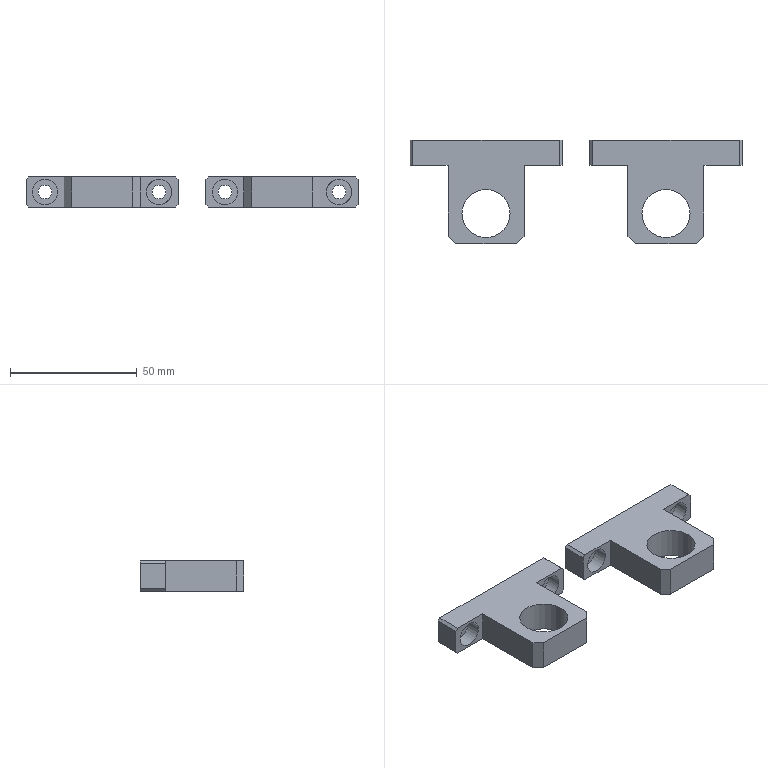Part | 2 solids | 46 faces | box 131 x 41 x 12 mm | volume 27460 mm3 | plane 36 | cylinder 10 | commonest cylinder face diameters 5.5 x4 10 x4 19 x2
STEP:
#1=CARTESIAN_POINT('',(22.5,18.2,5.));
#2=VERTEX_POINT('',#1);
#3=CARTESIAN_POINT('',(22.5,18.2,0.));
#4=DIRECTION('',(0.,-1.,0.));
#5=DIRECTION('',(0.,0.,1.));
#6=AXIS2_PLACEMENT_3D('',#3,#4,#5);
#7=CIRCLE('',#6,5.);
#8=EDGE_CURVE('',#2,#2,#7,.T.);
#9=ORIENTED_EDGE('',*,*,#8,.T.);
#10=EDGE_LOOP('',(#9));
#11=FACE_BOUND('',#10,.T.);
#12=CARTESIAN_POINT('',(22.5,18.2,2.75));
#13=VERTEX_POINT('',#12);
#14=CARTESIAN_POINT('',(22.5,18.2,0.));
#15=DIRECTION('',(0.,-1.,0.));
#16=DIRECTION('',(0.,0.,1.));
#17=AXIS2_PLACEMENT_3D('',#14,#15,#16);
#18=CIRCLE('',#17,2.75);
#19=EDGE_CURVE('',#13,#13,#18,.T.);
#20=ORIENTED_EDGE('',*,*,#19,.F.);
#21=EDGE_LOOP('',(#20));
#22=FACE_BOUND('',#21,.T.);
#23=CARTESIAN_POINT('',(-19.75,18.2,0.));
#24=DIRECTION('',(0.,1.,0.));
#25=DIRECTION('',(0.,0.,1.));
#26=AXIS2_PLACEMENT_3D('',#23,#24,#25);
#27=PLANE('',#26);
#28=ADVANCED_FACE('',(#11,#22),#27,.F.);
#29=CARTESIAN_POINT('',(-22.5,18.2,-5.));
#30=VERTEX_POINT('',#29);
#31=CARTESIAN_POINT('',(-22.5,18.2,0.));
#32=DIRECTION('',(0.,-1.,0.));
#33=DIRECTION('',(0.,0.,-1.));
#34=AXIS2_PLACEMENT_3D('',#31,#32,#33);
#35=CIRCLE('',#34,5.);
#36=EDGE_CURVE('',#30,#30,#35,.T.);
#37=ORIENTED_EDGE('',*,*,#36,.T.);
#38=EDGE_LOOP('',(#37));
#39=FACE_BOUND('',#38,.T.);
#40=CARTESIAN_POINT('',(-22.5,18.2,-2.75));
#41=VERTEX_POINT('',#40);
#42=CARTESIAN_POINT('',(-22.5,18.2,0.));
#43=DIRECTION('',(0.,-1.,0.));
#44=DIRECTION('',(0.,0.,-1.));
#45=AXIS2_PLACEMENT_3D('',#42,#43,#44);
#46=CIRCLE('',#45,2.75);
#47=EDGE_CURVE('',#41,#41,#46,.T.);
#48=ORIENTED_EDGE('',*,*,#47,.F.);
#49=EDGE_LOOP('',(#48));
#50=FACE_BOUND('',#49,.T.);
#51=CARTESIAN_POINT('',(-19.75,18.2,0.));
#52=DIRECTION('',(0.,1.,0.));
#53=DIRECTION('',(0.,0.,1.));
#54=AXIS2_PLACEMENT_3D('',#51,#52,#53);
#55=PLANE('',#54);
#56=ADVANCED_FACE('',(#39,#50),#55,.F.);
#57=CARTESIAN_POINT('',(29.,12.5,-6.));
#58=VERTEX_POINT('',#57);
#59=CARTESIAN_POINT('',(30.,12.5,-5.));
#60=VERTEX_POINT('',#59);
#61=CARTESIAN_POINT('',(5.5,12.5,-29.5));
#62=DIRECTION('',(0.7071,0.,0.7071));
#63=VECTOR('',#62,1000.);
#64=LINE('',#61,#63);
#65=EDGE_CURVE('',#58,#60,#64,.T.);
#66=ORIENTED_EDGE('',*,*,#65,.F.);
#67=CARTESIAN_POINT('',(29.,22.5,-6.));
#68=VERTEX_POINT('',#67);
#69=CARTESIAN_POINT('',(29.,0.,-6.));
#70=DIRECTION('',(0.,-1.,0.));
#71=VECTOR('',#70,1000.);
#72=LINE('',#69,#71);
#73=EDGE_CURVE('',#68,#58,#72,.T.);
#74=ORIENTED_EDGE('',*,*,#73,.F.);
#75=CARTESIAN_POINT('',(30.,22.5,-5.));
#76=VERTEX_POINT('',#75);
#77=CARTESIAN_POINT('',(30.,22.5,-5.));
#78=DIRECTION('',(-0.7071,0.,-0.7071));
#79=VECTOR('',#78,1000.);
#80=LINE('',#77,#79);
#81=EDGE_CURVE('',#76,#68,#80,.T.);
#82=ORIENTED_EDGE('',*,*,#81,.F.);
#83=CARTESIAN_POINT('',(30.,22.5,-5.));
#84=DIRECTION('',(0.,1.,0.));
#85=VECTOR('',#84,1000.);
#86=LINE('',#83,#85);
#87=EDGE_CURVE('',#60,#76,#86,.T.);
#88=ORIENTED_EDGE('',*,*,#87,.F.);
#89=EDGE_LOOP('',(#66,#74,#82,#88));
#90=FACE_BOUND('',#89,.T.);
#91=CARTESIAN_POINT('',(30.,22.5,-5.));
#92=DIRECTION('',(-0.7071,0.,0.7071));
#93=DIRECTION('',(0.,1.,0.));
#94=AXIS2_PLACEMENT_3D('',#91,#92,#93);
#95=PLANE('',#94);
#96=ADVANCED_FACE('',(#90),#95,.F.);
#97=CARTESIAN_POINT('',(30.,12.5,5.));
#98=VERTEX_POINT('',#97);
#99=CARTESIAN_POINT('',(29.,12.5,6.));
#100=VERTEX_POINT('',#99);
#101=CARTESIAN_POINT('',(-0.5,12.5,35.5));
#102=DIRECTION('',(-0.7071,0.,0.7071));
#103=VECTOR('',#102,1000.);
#104=LINE('',#101,#103);
#105=EDGE_CURVE('',#98,#100,#104,.T.);
#106=ORIENTED_EDGE('',*,*,#105,.F.);
#107=CARTESIAN_POINT('',(30.,22.5,5.));
#108=VERTEX_POINT('',#107);
#109=CARTESIAN_POINT('',(30.,12.5,5.));
#110=DIRECTION('',(0.,-1.,0.));
#111=VECTOR('',#110,1000.);
#112=LINE('',#109,#111);
#113=EDGE_CURVE('',#108,#98,#112,.T.);
#114=ORIENTED_EDGE('',*,*,#113,.F.);
#115=CARTESIAN_POINT('',(29.,22.5,6.));
#116=VERTEX_POINT('',#115);
#117=CARTESIAN_POINT('',(29.,22.5,6.));
#118=DIRECTION('',(0.7071,0.,-0.7071));
#119=VECTOR('',#118,1000.);
#120=LINE('',#117,#119);
#121=EDGE_CURVE('',#116,#108,#120,.T.);
#122=ORIENTED_EDGE('',*,*,#121,.F.);
#123=CARTESIAN_POINT('',(29.,22.5,6.));
#124=DIRECTION('',(0.,1.,0.));
#125=VECTOR('',#124,1000.);
#126=LINE('',#123,#125);
#127=EDGE_CURVE('',#100,#116,#126,.T.);
#128=ORIENTED_EDGE('',*,*,#127,.F.);
#129=EDGE_LOOP('',(#106,#114,#122,#128));
#130=FACE_BOUND('',#129,.T.);
#131=CARTESIAN_POINT('',(29.,0.,6.));
#132=DIRECTION('',(0.7071,0.,0.7071));
#133=DIRECTION('',(0.,-1.,0.));
#134=AXIS2_PLACEMENT_3D('',#131,#132,#133);
#135=PLANE('',#134);
#136=ADVANCED_FACE('',(#130),#135,.T.);
#137=CARTESIAN_POINT('',(-29.,22.5,-6.));
#138=VERTEX_POINT('',#137);
#139=CARTESIAN_POINT('',(-30.,22.5,-5.));
#140=VERTEX_POINT('',#139);
#141=CARTESIAN_POINT('',(-30.,22.5,-5.));
#142=DIRECTION('',(-0.7071,0.,0.7071));
#143=VECTOR('',#142,1000.);
#144=LINE('',#141,#143);
#145=EDGE_CURVE('',#138,#140,#144,.T.);
#146=ORIENTED_EDGE('',*,*,#145,.F.);
#147=CARTESIAN_POINT('',(-29.,12.5,-6.));
#148=VERTEX_POINT('',#147);
#149=CARTESIAN_POINT('',(-29.,0.,-6.));
#150=DIRECTION('',(0.,1.,0.));
#151=VECTOR('',#150,1000.);
#152=LINE('',#149,#151);
#153=EDGE_CURVE('',#148,#138,#152,.T.);
#154=ORIENTED_EDGE('',*,*,#153,.F.);
#155=CARTESIAN_POINT('',(-30.,12.5,-5.));
#156=VERTEX_POINT('',#155);
#157=CARTESIAN_POINT('',(-30.,12.5,-5.));
#158=DIRECTION('',(0.7071,0.,-0.7071));
#159=VECTOR('',#158,1000.);
#160=LINE('',#157,#159);
#161=EDGE_CURVE('',#156,#148,#160,.T.);
#162=ORIENTED_EDGE('',*,*,#161,.F.);
#163=CARTESIAN_POINT('',(-30.,22.5,-5.));
#164=DIRECTION('',(0.,-1.,0.));
#165=VECTOR('',#164,1000.);
#166=LINE('',#163,#165);
#167=EDGE_CURVE('',#140,#156,#166,.T.);
#168=ORIENTED_EDGE('',*,*,#167,.F.);
#169=EDGE_LOOP('',(#146,#154,#162,#168));
#170=FACE_BOUND('',#169,.T.);
#171=CARTESIAN_POINT('',(-30.,22.5,-5.));
#172=DIRECTION('',(0.7071,0.,0.7071));
#173=DIRECTION('',(0.,-1.,0.));
#174=AXIS2_PLACEMENT_3D('',#171,#172,#173);
#175=PLANE('',#174);
#176=ADVANCED_FACE('',(#170),#175,.F.);
#177=CARTESIAN_POINT('',(-30.,22.5,5.));
#178=VERTEX_POINT('',#177);
#179=CARTESIAN_POINT('',(-29.,22.5,6.));
#180=VERTEX_POINT('',#179);
#181=CARTESIAN_POINT('',(-29.,22.5,6.));
#182=DIRECTION('',(0.7071,0.,0.7071));
#183=VECTOR('',#182,1000.);
#184=LINE('',#181,#183);
#185=EDGE_CURVE('',#178,#180,#184,.T.);
#186=ORIENTED_EDGE('',*,*,#185,.F.);
#187=CARTESIAN_POINT('',(-30.,12.5,5.));
#188=VERTEX_POINT('',#187);
#189=CARTESIAN_POINT('',(-30.,22.5,5.));
#190=DIRECTION('',(0.,1.,0.));
#191=VECTOR('',#190,1000.);
#192=LINE('',#189,#191);
#193=EDGE_CURVE('',#188,#178,#192,.T.);
#194=ORIENTED_EDGE('',*,*,#193,.F.);
#195=CARTESIAN_POINT('',(-29.,12.5,6.));
#196=VERTEX_POINT('',#195);
#197=CARTESIAN_POINT('',(-29.,12.5,6.));
#198=DIRECTION('',(-0.7071,0.,-0.7071));
#199=VECTOR('',#198,1000.);
#200=LINE('',#197,#199);
#201=EDGE_CURVE('',#196,#188,#200,.T.);
#202=ORIENTED_EDGE('',*,*,#201,.F.);
#203=CARTESIAN_POINT('',(-29.,12.5,6.));
#204=DIRECTION('',(0.,-1.,0.));
#205=VECTOR('',#204,1000.);
#206=LINE('',#203,#205);
#207=EDGE_CURVE('',#180,#196,#206,.T.);
#208=ORIENTED_EDGE('',*,*,#207,.F.);
#209=EDGE_LOOP('',(#186,#194,#202,#208));
#210=FACE_BOUND('',#209,.T.);
#211=CARTESIAN_POINT('',(-29.,0.,6.));
#212=DIRECTION('',(-0.7071,0.,0.7071));
#213=DIRECTION('',(0.,1.,0.));
#214=AXIS2_PLACEMENT_3D('',#211,#212,#213);
#215=PLANE('',#214);
#216=ADVANCED_FACE('',(#210),#215,.T.);
#217=CARTESIAN_POINT('',(12.,-18.5,6.));
#218=VERTEX_POINT('',#217);
#219=CARTESIAN_POINT('',(15.,-15.5,6.));
#220=VERTEX_POINT('',#219);
#221=CARTESIAN_POINT('',(17.25,-13.25,6.));
#222=DIRECTION('',(0.7071,0.7071,0.));
#223=VECTOR('',#222,1000.);
#224=LINE('',#221,#223);
#225=EDGE_CURVE('',#218,#220,#224,.T.);
#226=ORIENTED_EDGE('',*,*,#225,.F.);
#227=CARTESIAN_POINT('',(12.,-18.5,-6.));
#228=VERTEX_POINT('',#227);
#229=CARTESIAN_POINT('',(12.,-18.5,6.));
#230=DIRECTION('',(0.,0.,1.));
#231=VECTOR('',#230,1000.);
#232=LINE('',#229,#231);
#233=EDGE_CURVE('',#228,#218,#232,.T.);
#234=ORIENTED_EDGE('',*,*,#233,.F.);
#235=CARTESIAN_POINT('',(15.,-15.5,-6.));
#236=VERTEX_POINT('',#235);
#237=CARTESIAN_POINT('',(15.,-15.5,-6.));
#238=DIRECTION('',(-0.7071,-0.7071,0.));
#239=VECTOR('',#238,1000.);
#240=LINE('',#237,#239);
#241=EDGE_CURVE('',#236,#228,#240,.T.);
#242=ORIENTED_EDGE('',*,*,#241,.F.);
#243=CARTESIAN_POINT('',(15.,-15.5,6.));
#244=DIRECTION('',(0.,0.,-1.));
#245=VECTOR('',#244,1000.);
#246=LINE('',#243,#245);
#247=EDGE_CURVE('',#220,#236,#246,.T.);
#248=ORIENTED_EDGE('',*,*,#247,.F.);
#249=EDGE_LOOP('',(#226,#234,#242,#248));
#250=FACE_BOUND('',#249,.T.);
#251=CARTESIAN_POINT('',(15.,-15.5,6.));
#252=DIRECTION('',(-0.7071,0.7071,0.));
#253=DIRECTION('',(0.,0.,-1.));
#254=AXIS2_PLACEMENT_3D('',#251,#252,#253);
#255=PLANE('',#254);
#256=ADVANCED_FACE('',(#250),#255,.F.);
#257=CARTESIAN_POINT('',(-15.,-15.5,6.));
#258=VERTEX_POINT('',#257);
#259=CARTESIAN_POINT('',(-12.,-18.5,6.));
#260=VERTEX_POINT('',#259);
#261=CARTESIAN_POINT('',(-17.25,-13.25,6.));
#262=DIRECTION('',(0.7071,-0.7071,0.));
#263=VECTOR('',#262,1000.);
#264=LINE('',#261,#263);
#265=EDGE_CURVE('',#258,#260,#264,.T.);
#266=ORIENTED_EDGE('',*,*,#265,.F.);
#267=CARTESIAN_POINT('',(-15.,-15.5,-6.));
#268=VERTEX_POINT('',#267);
#269=CARTESIAN_POINT('',(-15.,-15.5,6.));
#270=DIRECTION('',(0.,0.,1.));
#271=VECTOR('',#270,1000.);
#272=LINE('',#269,#271);
#273=EDGE_CURVE('',#268,#258,#272,.T.);
#274=ORIENTED_EDGE('',*,*,#273,.F.);
#275=CARTESIAN_POINT('',(-12.,-18.5,-6.));
#276=VERTEX_POINT('',#275);
#277=CARTESIAN_POINT('',(-12.,-18.5,-6.));
#278=DIRECTION('',(-0.7071,0.7071,0.));
#279=VECTOR('',#278,1000.);
#280=LINE('',#277,#279);
#281=EDGE_CURVE('',#276,#268,#280,.T.);
#282=ORIENTED_EDGE('',*,*,#281,.F.);
#283=CARTESIAN_POINT('',(-12.,-18.5,6.));
#284=DIRECTION('',(0.,0.,-1.));
#285=VECTOR('',#284,1000.);
#286=LINE('',#283,#285);
#287=EDGE_CURVE('',#260,#276,#286,.T.);
#288=ORIENTED_EDGE('',*,*,#287,.F.);
#289=EDGE_LOOP('',(#266,#274,#282,#288));
#290=FACE_BOUND('',#289,.T.);
#291=CARTESIAN_POINT('',(-12.,-18.5,6.));
#292=DIRECTION('',(0.7071,0.7071,0.));
#293=DIRECTION('',(0.,0.,-1.));
#294=AXIS2_PLACEMENT_3D('',#291,#292,#293);
#295=PLANE('',#294);
#296=ADVANCED_FACE('',(#290),#295,.F.);
#297=CARTESIAN_POINT('',(15.,12.5,6.));
#298=VERTEX_POINT('',#297);
#299=CARTESIAN_POINT('',(15.,-22.5,6.));
#300=DIRECTION('',(0.,1.,0.));
#301=VECTOR('',#300,1000.);
#302=LINE('',#299,#301);
#303=EDGE_CURVE('',#220,#298,#302,.T.);
#304=ORIENTED_EDGE('',*,*,#303,.F.);
#305=ORIENTED_EDGE('',*,*,#247,.T.);
#306=CARTESIAN_POINT('',(15.,12.5,-6.));
#307=VERTEX_POINT('',#306);
#308=CARTESIAN_POINT('',(15.,-22.5,-6.));
#309=DIRECTION('',(0.,1.,0.));
#310=VECTOR('',#309,1000.);
#311=LINE('',#308,#310);
#312=EDGE_CURVE('',#236,#307,#311,.T.);
#313=ORIENTED_EDGE('',*,*,#312,.T.);
#314=CARTESIAN_POINT('',(15.,12.5,6.));
#315=DIRECTION('',(0.,0.,-1.));
#316=VECTOR('',#315,1000.);
#317=LINE('',#314,#316);
#318=EDGE_CURVE('',#298,#307,#317,.T.);
#319=ORIENTED_EDGE('',*,*,#318,.F.);
#320=EDGE_LOOP('',(#304,#305,#313,#319));
#321=FACE_BOUND('',#320,.T.);
#322=CARTESIAN_POINT('',(15.,-22.5,6.));
#323=DIRECTION('',(-1.,0.,0.));
#324=DIRECTION('',(0.,0.,1.));
#325=AXIS2_PLACEMENT_3D('',#322,#323,#324);
#326=PLANE('',#325);
#327=ADVANCED_FACE('',(#321),#326,.F.);
#328=CARTESIAN_POINT('',(30.,12.5,6.));
#329=DIRECTION('',(0.,0.,-1.));
#330=VECTOR('',#329,1000.);
#331=LINE('',#328,#330);
#332=EDGE_CURVE('',#98,#60,#331,.T.);
#333=ORIENTED_EDGE('',*,*,#332,.F.);
#334=ORIENTED_EDGE('',*,*,#105,.T.);
#335=CARTESIAN_POINT('',(0.,12.5,6.));
#336=DIRECTION('',(1.,0.,0.));
#337=VECTOR('',#336,1000.);
#338=LINE('',#335,#337);
#339=EDGE_CURVE('',#298,#100,#338,.T.);
#340=ORIENTED_EDGE('',*,*,#339,.F.);
#341=ORIENTED_EDGE('',*,*,#318,.T.);
#342=CARTESIAN_POINT('',(-30.,12.5,-6.));
#343=DIRECTION('',(1.,0.,0.));
#344=VECTOR('',#343,1000.);
#345=LINE('',#342,#344);
#346=EDGE_CURVE('',#307,#58,#345,.T.);
#347=ORIENTED_EDGE('',*,*,#346,.T.);
#348=ORIENTED_EDGE('',*,*,#65,.T.);
#349=EDGE_LOOP('',(#333,#334,#340,#341,#347,#348));
#350=FACE_BOUND('',#349,.T.);
#351=CARTESIAN_POINT('',(17.5,12.5,0.));
#352=VERTEX_POINT('',#351);
#353=CARTESIAN_POINT('',(22.5,12.5,0.));
#354=DIRECTION('',(0.,-1.,0.));
#355=DIRECTION('',(-1.,0.,0.));
#356=AXIS2_PLACEMENT_3D('',#353,#354,#355);
#357=CIRCLE('',#356,5.);
#358=EDGE_CURVE('',#352,#352,#357,.T.);
#359=ORIENTED_EDGE('',*,*,#358,.F.);
#360=EDGE_LOOP('',(#359));
#361=FACE_BOUND('',#360,.T.);
#362=CARTESIAN_POINT('',(-30.,12.5,6.));
#363=DIRECTION('',(0.,1.,0.));
#364=DIRECTION('',(-1.,0.,0.));
#365=AXIS2_PLACEMENT_3D('',#362,#363,#364);
#366=PLANE('',#365);
#367=ADVANCED_FACE('',(#350,#361),#366,.F.);
#368=CARTESIAN_POINT('',(-15.,12.5,6.));
#369=VERTEX_POINT('',#368);
#370=CARTESIAN_POINT('',(-30.,12.5,6.));
#371=DIRECTION('',(1.,0.,0.));
#372=VECTOR('',#371,1000.);
#373=LINE('',#370,#372);
#374=EDGE_CURVE('',#196,#369,#373,.T.);
#375=ORIENTED_EDGE('',*,*,#374,.F.);
#376=ORIENTED_EDGE('',*,*,#201,.T.);
#377=CARTESIAN_POINT('',(-30.,12.5,6.));
#378=DIRECTION('',(0.,0.,-1.));
#379=VECTOR('',#378,1000.);
#380=LINE('',#377,#379);
#381=EDGE_CURVE('',#188,#156,#380,.T.);
#382=ORIENTED_EDGE('',*,*,#381,.T.);
#383=ORIENTED_EDGE('',*,*,#161,.T.);
#384=CARTESIAN_POINT('',(-15.,12.5,-6.));
#385=VERTEX_POINT('',#384);
#386=CARTESIAN_POINT('',(-30.,12.5,-6.));
#387=DIRECTION('',(1.,0.,0.));
#388=VECTOR('',#387,1000.);
#389=LINE('',#386,#388);
#390=EDGE_CURVE('',#148,#385,#389,.T.);
#391=ORIENTED_EDGE('',*,*,#390,.T.);
#392=CARTESIAN_POINT('',(-15.,12.5,6.));
#393=DIRECTION('',(0.,0.,-1.));
#394=VECTOR('',#393,1000.);
#395=LINE('',#392,#394);
#396=EDGE_CURVE('',#369,#385,#395,.T.);
#397=ORIENTED_EDGE('',*,*,#396,.F.);
#398=EDGE_LOOP('',(#375,#376,#382,#383,#391,#397));
#399=FACE_BOUND('',#398,.T.);
#400=CARTESIAN_POINT('',(-22.5,12.5,-5.));
#401=VERTEX_POINT('',#400);
#402=CARTESIAN_POINT('',(-22.5,12.5,0.));
#403=DIRECTION('',(0.,-1.,0.));
#404=DIRECTION('',(0.,0.,-1.));
#405=AXIS2_PLACEMENT_3D('',#402,#403,#404);
#406=CIRCLE('',#405,5.);
#407=EDGE_CURVE('',#401,#401,#406,.T.);
#408=ORIENTED_EDGE('',*,*,#407,.F.);
#409=EDGE_LOOP('',(#408));
#410=FACE_BOUND('',#409,.T.);
#411=CARTESIAN_POINT('',(-30.,12.5,6.));
#412=DIRECTION('',(0.,1.,0.));
#413=DIRECTION('',(-1.,0.,0.));
#414=AXIS2_PLACEMENT_3D('',#411,#412,#413);
#415=PLANE('',#414);
#416=ADVANCED_FACE('',(#399,#410),#415,.F.);
#417=CARTESIAN_POINT('',(-15.,-22.5,-6.));
#418=DIRECTION('',(0.,-1.,0.));
#419=VECTOR('',#418,1000.);
#420=LINE('',#417,#419);
#421=EDGE_CURVE('',#385,#268,#420,.T.);
#422=ORIENTED_EDGE('',*,*,#421,.T.);
#423=ORIENTED_EDGE('',*,*,#273,.T.);
#424=CARTESIAN_POINT('',(-15.,-22.5,6.));
#425=DIRECTION('',(0.,-1.,0.));
#426=VECTOR('',#425,1000.);
#427=LINE('',#424,#426);
#428=EDGE_CURVE('',#369,#258,#427,.T.);
#429=ORIENTED_EDGE('',*,*,#428,.F.);
#430=ORIENTED_EDGE('',*,*,#396,.T.);
#431=EDGE_LOOP('',(#422,#423,#429,#430));
#432=FACE_BOUND('',#431,.T.);
#433=CARTESIAN_POINT('',(-15.,-22.5,6.));
#434=DIRECTION('',(1.,0.,0.));
#435=DIRECTION('',(0.,0.,-1.));
#436=AXIS2_PLACEMENT_3D('',#433,#434,#435);
#437=PLANE('',#436);
#438=ADVANCED_FACE('',(#432),#437,.F.);
#439=ORIENTED_EDGE('',*,*,#390,.F.);
#440=ORIENTED_EDGE('',*,*,#153,.T.);
#441=CARTESIAN_POINT('',(-30.,22.5,-6.));
#442=DIRECTION('',(-1.,0.,0.));
#443=VECTOR('',#442,1000.);
#444=LINE('',#441,#443);
#445=EDGE_CURVE('',#68,#138,#444,.T.);
#446=ORIENTED_EDGE('',*,*,#445,.F.);
#447=ORIENTED_EDGE('',*,*,#73,.T.);
#448=ORIENTED_EDGE('',*,*,#346,.F.);
#449=ORIENTED_EDGE('',*,*,#312,.F.);
#450=ORIENTED_EDGE('',*,*,#241,.T.);
#451=CARTESIAN_POINT('',(-30.,-18.5,-6.));
#452=DIRECTION('',(1.,0.,0.));
#453=VECTOR('',#452,1000.);
#454=LINE('',#451,#453);
#455=EDGE_CURVE('',#276,#228,#454,.T.);
#456=ORIENTED_EDGE('',*,*,#455,.F.);
#457=ORIENTED_EDGE('',*,*,#281,.T.);
#458=ORIENTED_EDGE('',*,*,#421,.F.);
#459=EDGE_LOOP('',(#439,#440,#446,#447,#448,#449,#450,#456,#457,#458));
#460=FACE_BOUND('',#459,.T.);
#461=CARTESIAN_POINT('',(-9.5,-6.5,-6.));
#462=VERTEX_POINT('',#461);
#463=CARTESIAN_POINT('',(0.,-6.5,-6.));
#464=DIRECTION('',(0.,0.,-1.));
#465=DIRECTION('',(-1.,0.,0.));
#466=AXIS2_PLACEMENT_3D('',#463,#464,#465);
#467=CIRCLE('',#466,9.5);
#468=EDGE_CURVE('',#462,#462,#467,.T.);
#469=ORIENTED_EDGE('',*,*,#468,.F.);
#470=EDGE_LOOP('',(#469));
#471=FACE_BOUND('',#470,.T.);
#472=CARTESIAN_POINT('',(0.,0.,-6.));
#473=DIRECTION('',(0.,0.,1.));
#474=DIRECTION('',(1.,0.,0.));
#475=AXIS2_PLACEMENT_3D('',#472,#473,#474);
#476=PLANE('',#475);
#477=ADVANCED_FACE('',(#460,#471),#476,.F.);
#478=CARTESIAN_POINT('',(-9.5,-6.5,6.));
#479=VERTEX_POINT('',#478);
#480=CARTESIAN_POINT('',(0.,-6.5,6.));
#481=DIRECTION('',(0.,0.,-1.));
#482=DIRECTION('',(-1.,0.,0.));
#483=AXIS2_PLACEMENT_3D('',#480,#481,#482);
#484=CIRCLE('',#483,9.5);
#485=EDGE_CURVE('',#479,#479,#484,.T.);
#486=ORIENTED_EDGE('',*,*,#485,.T.);
#487=EDGE_LOOP('',(#486));
#488=FACE_BOUND('',#487,.T.);
#489=CARTESIAN_POINT('',(-30.,22.5,6.));
#490=DIRECTION('',(-1.,0.,0.));
#491=VECTOR('',#490,1000.);
#492=LINE('',#489,#491);
#493=EDGE_CURVE('',#116,#180,#492,.T.);
#494=ORIENTED_EDGE('',*,*,#493,.T.);
#495=ORIENTED_EDGE('',*,*,#207,.T.);
#496=ORIENTED_EDGE('',*,*,#374,.T.);
#497=ORIENTED_EDGE('',*,*,#428,.T.);
#498=ORIENTED_EDGE('',*,*,#265,.T.);
#499=CARTESIAN_POINT('',(-30.,-18.5,6.));
#500=DIRECTION('',(1.,0.,0.));
#501=VECTOR('',#500,1000.);
#502=LINE('',#499,#501);
#503=EDGE_CURVE('',#260,#218,#502,.T.);
#504=ORIENTED_EDGE('',*,*,#503,.T.);
#505=ORIENTED_EDGE('',*,*,#225,.T.);
#506=ORIENTED_EDGE('',*,*,#303,.T.);
#507=ORIENTED_EDGE('',*,*,#339,.T.);
#508=ORIENTED_EDGE('',*,*,#127,.T.);
#509=EDGE_LOOP('',(#494,#495,#496,#497,#498,#504,#505,#506,#507,#508));
#510=FACE_BOUND('',#509,.T.);
#511=CARTESIAN_POINT('',(0.,0.,6.));
#512=DIRECTION('',(0.,0.,1.));
#513=DIRECTION('',(1.,0.,0.));
#514=AXIS2_PLACEMENT_3D('',#511,#512,#513);
#515=PLANE('',#514);
#516=ADVANCED_FACE('',(#488,#510),#515,.T.);
#517=ORIENTED_EDGE('',*,*,#503,.F.);
#518=ORIENTED_EDGE('',*,*,#287,.T.);
#519=ORIENTED_EDGE('',*,*,#455,.T.);
#520=ORIENTED_EDGE('',*,*,#233,.T.);
#521=EDGE_LOOP('',(#517,#518,#519,#520));
#522=FACE_BOUND('',#521,.T.);
#523=CARTESIAN_POINT('',(-30.,-18.5,6.));
#524=DIRECTION('',(0.,1.,0.));
#525=DIRECTION('',(0.,0.,1.));
#526=AXIS2_PLACEMENT_3D('',#523,#524,#525);
#527=PLANE('',#526);
#528=ADVANCED_FACE('',(#522),#527,.F.);
#529=ORIENTED_EDGE('',*,*,#381,.F.);
#530=ORIENTED_EDGE('',*,*,#193,.T.);
#531=CARTESIAN_POINT('',(-30.,22.5,6.));
#532=DIRECTION('',(0.,0.,-1.));
#533=VECTOR('',#532,1000.);
#534=LINE('',#531,#533);
#535=EDGE_CURVE('',#178,#140,#534,.T.);
#536=ORIENTED_EDGE('',*,*,#535,.T.);
#537=ORIENTED_EDGE('',*,*,#167,.T.);
#538=EDGE_LOOP('',(#529,#530,#536,#537));
#539=FACE_BOUND('',#538,.T.);
#540=CARTESIAN_POINT('',(-30.,22.5,6.));
#541=DIRECTION('',(1.,0.,0.));
#542=DIRECTION('',(0.,1.,0.));
#543=AXIS2_PLACEMENT_3D('',#540,#541,#542);
#544=PLANE('',#543);
#545=ADVANCED_FACE('',(#539),#544,.F.);
#546=ORIENTED_EDGE('',*,*,#535,.F.);
#547=ORIENTED_EDGE('',*,*,#185,.T.);
#548=ORIENTED_EDGE('',*,*,#493,.F.);
#549=ORIENTED_EDGE('',*,*,#121,.T.);
#550=CARTESIAN_POINT('',(30.,22.5,6.));
#551=DIRECTION('',(0.,0.,-1.));
#552=VECTOR('',#551,1000.);
#553=LINE('',#550,#552);
#554=EDGE_CURVE('',#108,#76,#553,.T.);
#555=ORIENTED_EDGE('',*,*,#554,.T.);
#556=ORIENTED_EDGE('',*,*,#81,.T.);
#557=ORIENTED_EDGE('',*,*,#445,.T.);
#558=ORIENTED_EDGE('',*,*,#145,.T.);
#559=EDGE_LOOP('',(#546,#547,#548,#549,#555,#556,#557,#558));
#560=FACE_BOUND('',#559,.T.);
#561=CARTESIAN_POINT('',(-22.5,22.5,-2.75));
#562=VERTEX_POINT('',#561);
#563=CARTESIAN_POINT('',(-22.5,22.5,0.));
#564=DIRECTION('',(0.,-1.,0.));
#565=DIRECTION('',(0.,0.,-1.));
#566=AXIS2_PLACEMENT_3D('',#563,#564,#565);
#567=CIRCLE('',#566,2.75);
#568=EDGE_CURVE('',#562,#562,#567,.T.);
#569=ORIENTED_EDGE('',*,*,#568,.T.);
#570=EDGE_LOOP('',(#569));
#571=FACE_BOUND('',#570,.T.);
#572=CARTESIAN_POINT('',(22.5,22.5,-2.75));
#573=VERTEX_POINT('',#572);
#574=CARTESIAN_POINT('',(22.5,22.5,0.));
#575=DIRECTION('',(0.,-1.,0.));
#576=DIRECTION('',(0.,0.,-1.));
#577=AXIS2_PLACEMENT_3D('',#574,#575,#576);
#578=CIRCLE('',#577,2.75);
#579=EDGE_CURVE('',#573,#573,#578,.T.);
#580=ORIENTED_EDGE('',*,*,#579,.T.);
#581=EDGE_LOOP('',(#580));
#582=FACE_BOUND('',#581,.T.);
#583=CARTESIAN_POINT('',(-30.,22.5,6.));
#584=DIRECTION('',(0.,-1.,0.));
#585=DIRECTION('',(0.,0.,-1.));
#586=AXIS2_PLACEMENT_3D('',#583,#584,#585);
#587=PLANE('',#586);
#588=ADVANCED_FACE('',(#560,#571,#582),#587,.F.);
#589=ORIENTED_EDGE('',*,*,#554,.F.);
#590=ORIENTED_EDGE('',*,*,#113,.T.);
#591=ORIENTED_EDGE('',*,*,#332,.T.);
#592=ORIENTED_EDGE('',*,*,#87,.T.);
#593=EDGE_LOOP('',(#589,#590,#591,#592));
#594=FACE_BOUND('',#593,.T.);
#595=CARTESIAN_POINT('',(30.,22.5,6.));
#596=DIRECTION('',(-1.,0.,0.));
#597=DIRECTION('',(0.,-1.,0.));
#598=AXIS2_PLACEMENT_3D('',#595,#596,#597);
#599=PLANE('',#598);
#600=ADVANCED_FACE('',(#594),#599,.F.);
#601=ORIENTED_EDGE('',*,*,#468,.T.);
#602=EDGE_LOOP('',(#601));
#603=FACE_BOUND('',#602,.T.);
#604=ORIENTED_EDGE('',*,*,#485,.F.);
#605=EDGE_LOOP('',(#604));
#606=FACE_BOUND('',#605,.T.);
#607=CARTESIAN_POINT('',(0.,-6.5,6.));
#608=DIRECTION('',(0.,0.,-1.));
#609=DIRECTION('',(-1.,0.,0.));
#610=AXIS2_PLACEMENT_3D('',#607,#608,#609);
#611=CYLINDRICAL_SURFACE('',#610,9.5);
#612=ADVANCED_FACE('',(#603,#606),#611,.F.);
#613=ORIENTED_EDGE('',*,*,#47,.T.);
#614=EDGE_LOOP('',(#613));
#615=FACE_BOUND('',#614,.T.);
#616=ORIENTED_EDGE('',*,*,#568,.F.);
#617=EDGE_LOOP('',(#616));
#618=FACE_BOUND('',#617,.T.);
#619=CARTESIAN_POINT('',(-22.5,12.5,0.));
#620=DIRECTION('',(0.,-1.,0.));
#621=DIRECTION('',(0.,0.,-1.));
#622=AXIS2_PLACEMENT_3D('',#619,#620,#621);
#623=CYLINDRICAL_SURFACE('',#622,2.75);
#624=ADVANCED_FACE('',(#615,#618),#623,.F.);
#625=ORIENTED_EDGE('',*,*,#407,.T.);
#626=EDGE_LOOP('',(#625));
#627=FACE_BOUND('',#626,.T.);
#628=ORIENTED_EDGE('',*,*,#36,.F.);
#629=EDGE_LOOP('',(#628));
#630=FACE_BOUND('',#629,.T.);
#631=CARTESIAN_POINT('',(-22.5,12.5,0.));
#632=DIRECTION('',(0.,-1.,0.));
#633=DIRECTION('',(0.,0.,-1.));
#634=AXIS2_PLACEMENT_3D('',#631,#632,#633);
#635=CYLINDRICAL_SURFACE('',#634,5.);
#636=ADVANCED_FACE('',(#627,#630),#635,.F.);
#637=ORIENTED_EDGE('',*,*,#19,.T.);
#638=EDGE_LOOP('',(#637));
#639=FACE_BOUND('',#638,.T.);
#640=ORIENTED_EDGE('',*,*,#579,.F.);
#641=EDGE_LOOP('',(#640));
#642=FACE_BOUND('',#641,.T.);
#643=CARTESIAN_POINT('',(22.5,12.5,0.));
#644=DIRECTION('',(0.,-1.,0.));
#645=DIRECTION('',(0.,0.,-1.));
#646=AXIS2_PLACEMENT_3D('',#643,#644,#645);
#647=CYLINDRICAL_SURFACE('',#646,2.75);
#648=ADVANCED_FACE('',(#639,#642),#647,.F.);
#649=ORIENTED_EDGE('',*,*,#358,.T.);
#650=EDGE_LOOP('',(#649));
#651=FACE_BOUND('',#650,.T.);
#652=ORIENTED_EDGE('',*,*,#8,.F.);
#653=EDGE_LOOP('',(#652));
#654=FACE_BOUND('',#653,.T.);
#655=CARTESIAN_POINT('',(22.5,12.5,0.));
#656=DIRECTION('',(0.,-1.,0.));
#657=DIRECTION('',(0.,0.,-1.));
#658=AXIS2_PLACEMENT_3D('',#655,#656,#657);
#659=CYLINDRICAL_SURFACE('',#658,5.);
#660=ADVANCED_FACE('',(#651,#654),#659,.F.);
#661=CLOSED_SHELL('',(#28,#56,#96,#136,#176,#216,#256,#296,#327,#367,#416,#438,#477,#516,#528,#545,#588,#600,#612,#624,#636,#648,#660));
#662=MANIFOLD_SOLID_BREP('',#661);
#663=CARTESIAN_POINT('',(-48.5,18.2,5.));
#664=VERTEX_POINT('',#663);
#665=CARTESIAN_POINT('',(-48.5,18.2,0.));
#666=DIRECTION('',(0.,-1.,0.));
#667=DIRECTION('',(0.,0.,1.));
#668=AXIS2_PLACEMENT_3D('',#665,#666,#667);
#669=CIRCLE('',#668,5.);
#670=EDGE_CURVE('',#664,#664,#669,.T.);
#671=ORIENTED_EDGE('',*,*,#670,.T.);
#672=EDGE_LOOP('',(#671));
#673=FACE_BOUND('',#672,.T.);
#674=CARTESIAN_POINT('',(-48.5,18.2,2.75));
#675=VERTEX_POINT('',#674);
#676=CARTESIAN_POINT('',(-48.5,18.2,0.));
#677=DIRECTION('',(0.,-1.,0.));
#678=DIRECTION('',(0.,0.,1.));
#679=AXIS2_PLACEMENT_3D('',#676,#677,#678);
#680=CIRCLE('',#679,2.75);
#681=EDGE_CURVE('',#675,#675,#680,.T.);
#682=ORIENTED_EDGE('',*,*,#681,.F.);
#683=EDGE_LOOP('',(#682));
#684=FACE_BOUND('',#683,.T.);
#685=CARTESIAN_POINT('',(-90.75,18.2,0.));
#686=DIRECTION('',(0.,1.,0.));
#687=DIRECTION('',(0.,0.,1.));
#688=AXIS2_PLACEMENT_3D('',#685,#686,#687);
#689=PLANE('',#688);
#690=ADVANCED_FACE('',(#673,#684),#689,.F.);
#691=CARTESIAN_POINT('',(-93.5,18.2,-5.));
#692=VERTEX_POINT('',#691);
#693=CARTESIAN_POINT('',(-93.5,18.2,0.));
#694=DIRECTION('',(0.,-1.,0.));
#695=DIRECTION('',(0.,0.,-1.));
#696=AXIS2_PLACEMENT_3D('',#693,#694,#695);
#697=CIRCLE('',#696,5.);
#698=EDGE_CURVE('',#692,#692,#697,.T.);
#699=ORIENTED_EDGE('',*,*,#698,.T.);
#700=EDGE_LOOP('',(#699));
#701=FACE_BOUND('',#700,.T.);
#702=CARTESIAN_POINT('',(-93.5,18.2,-2.75));
#703=VERTEX_POINT('',#702);
#704=CARTESIAN_POINT('',(-93.5,18.2,0.));
#705=DIRECTION('',(0.,-1.,0.));
#706=DIRECTION('',(0.,0.,-1.));
#707=AXIS2_PLACEMENT_3D('',#704,#705,#706);
#708=CIRCLE('',#707,2.75);
#709=EDGE_CURVE('',#703,#703,#708,.T.);
#710=ORIENTED_EDGE('',*,*,#709,.F.);
#711=EDGE_LOOP('',(#710));
#712=FACE_BOUND('',#711,.T.);
#713=CARTESIAN_POINT('',(-90.75,18.2,0.));
#714=DIRECTION('',(0.,1.,0.));
#715=DIRECTION('',(0.,0.,1.));
#716=AXIS2_PLACEMENT_3D('',#713,#714,#715);
#717=PLANE('',#716);
#718=ADVANCED_FACE('',(#701,#712),#717,.F.);
#719=CARTESIAN_POINT('',(-42.,12.5,-6.));
#720=VERTEX_POINT('',#719);
#721=CARTESIAN_POINT('',(-41.,12.5,-5.));
#722=VERTEX_POINT('',#721);
#723=CARTESIAN_POINT('',(-65.5,12.5,-29.5));
#724=DIRECTION('',(0.7071,0.,0.7071));
#725=VECTOR('',#724,1000.);
#726=LINE('',#723,#725);
#727=EDGE_CURVE('',#720,#722,#726,.T.);
#728=ORIENTED_EDGE('',*,*,#727,.F.);
#729=CARTESIAN_POINT('',(-42.,22.5,-6.));
#730=VERTEX_POINT('',#729);
#731=CARTESIAN_POINT('',(-42.,0.,-6.));
#732=DIRECTION('',(0.,-1.,0.));
#733=VECTOR('',#732,1000.);
#734=LINE('',#731,#733);
#735=EDGE_CURVE('',#730,#720,#734,.T.);
#736=ORIENTED_EDGE('',*,*,#735,.F.);
#737=CARTESIAN_POINT('',(-41.,22.5,-5.));
#738=VERTEX_POINT('',#737);
#739=CARTESIAN_POINT('',(-41.,22.5,-5.));
#740=DIRECTION('',(-0.7071,0.,-0.7071));
#741=VECTOR('',#740,1000.);
#742=LINE('',#739,#741);
#743=EDGE_CURVE('',#738,#730,#742,.T.);
#744=ORIENTED_EDGE('',*,*,#743,.F.);
#745=CARTESIAN_POINT('',(-41.,22.5,-5.));
#746=DIRECTION('',(0.,1.,0.));
#747=VECTOR('',#746,1000.);
#748=LINE('',#745,#747);
#749=EDGE_CURVE('',#722,#738,#748,.T.);
#750=ORIENTED_EDGE('',*,*,#749,.F.);
#751=EDGE_LOOP('',(#728,#736,#744,#750));
#752=FACE_BOUND('',#751,.T.);
#753=CARTESIAN_POINT('',(-41.,22.5,-5.));
#754=DIRECTION('',(-0.7071,0.,0.7071));
#755=DIRECTION('',(0.,1.,0.));
#756=AXIS2_PLACEMENT_3D('',#753,#754,#755);
#757=PLANE('',#756);
#758=ADVANCED_FACE('',(#752),#757,.F.);
#759=CARTESIAN_POINT('',(-41.,12.5,5.));
#760=VERTEX_POINT('',#759);
#761=CARTESIAN_POINT('',(-42.,12.5,6.));
#762=VERTEX_POINT('',#761);
#763=CARTESIAN_POINT('',(-71.5,12.5,35.5));
#764=DIRECTION('',(-0.7071,0.,0.7071));
#765=VECTOR('',#764,1000.);
#766=LINE('',#763,#765);
#767=EDGE_CURVE('',#760,#762,#766,.T.);
#768=ORIENTED_EDGE('',*,*,#767,.F.);
#769=CARTESIAN_POINT('',(-41.,22.5,5.));
#770=VERTEX_POINT('',#769);
#771=CARTESIAN_POINT('',(-41.,12.5,5.));
#772=DIRECTION('',(0.,-1.,0.));
#773=VECTOR('',#772,1000.);
#774=LINE('',#771,#773);
#775=EDGE_CURVE('',#770,#760,#774,.T.);
#776=ORIENTED_EDGE('',*,*,#775,.F.);
#777=CARTESIAN_POINT('',(-42.,22.5,6.));
#778=VERTEX_POINT('',#777);
#779=CARTESIAN_POINT('',(-42.,22.5,6.));
#780=DIRECTION('',(0.7071,0.,-0.7071));
#781=VECTOR('',#780,1000.);
#782=LINE('',#779,#781);
#783=EDGE_CURVE('',#778,#770,#782,.T.);
#784=ORIENTED_EDGE('',*,*,#783,.F.);
#785=CARTESIAN_POINT('',(-42.,22.5,6.));
#786=DIRECTION('',(0.,1.,0.));
#787=VECTOR('',#786,1000.);
#788=LINE('',#785,#787);
#789=EDGE_CURVE('',#762,#778,#788,.T.);
#790=ORIENTED_EDGE('',*,*,#789,.F.);
#791=EDGE_LOOP('',(#768,#776,#784,#790));
#792=FACE_BOUND('',#791,.T.);
#793=CARTESIAN_POINT('',(-42.,0.,6.));
#794=DIRECTION('',(0.7071,0.,0.7071));
#795=DIRECTION('',(0.,-1.,0.));
#796=AXIS2_PLACEMENT_3D('',#793,#794,#795);
#797=PLANE('',#796);
#798=ADVANCED_FACE('',(#792),#797,.T.);
#799=CARTESIAN_POINT('',(-100.,22.5,-6.));
#800=VERTEX_POINT('',#799);
#801=CARTESIAN_POINT('',(-101.,22.5,-5.));
#802=VERTEX_POINT('',#801);
#803=CARTESIAN_POINT('',(-101.,22.5,-5.));
#804=DIRECTION('',(-0.7071,0.,0.7071));
#805=VECTOR('',#804,1000.);
#806=LINE('',#803,#805);
#807=EDGE_CURVE('',#800,#802,#806,.T.);
#808=ORIENTED_EDGE('',*,*,#807,.F.);
#809=CARTESIAN_POINT('',(-100.,12.5,-6.));
#810=VERTEX_POINT('',#809);
#811=CARTESIAN_POINT('',(-100.,0.,-6.));
#812=DIRECTION('',(0.,1.,0.));
#813=VECTOR('',#812,1000.);
#814=LINE('',#811,#813);
#815=EDGE_CURVE('',#810,#800,#814,.T.);
#816=ORIENTED_EDGE('',*,*,#815,.F.);
#817=CARTESIAN_POINT('',(-101.,12.5,-5.));
#818=VERTEX_POINT('',#817);
#819=CARTESIAN_POINT('',(-101.,12.5,-5.));
#820=DIRECTION('',(0.7071,0.,-0.7071));
#821=VECTOR('',#820,1000.);
#822=LINE('',#819,#821);
#823=EDGE_CURVE('',#818,#810,#822,.T.);
#824=ORIENTED_EDGE('',*,*,#823,.F.);
#825=CARTESIAN_POINT('',(-101.,22.5,-5.));
#826=DIRECTION('',(0.,-1.,0.));
#827=VECTOR('',#826,1000.);
#828=LINE('',#825,#827);
#829=EDGE_CURVE('',#802,#818,#828,.T.);
#830=ORIENTED_EDGE('',*,*,#829,.F.);
#831=EDGE_LOOP('',(#808,#816,#824,#830));
#832=FACE_BOUND('',#831,.T.);
#833=CARTESIAN_POINT('',(-101.,22.5,-5.));
#834=DIRECTION('',(0.7071,0.,0.7071));
#835=DIRECTION('',(0.,-1.,0.));
#836=AXIS2_PLACEMENT_3D('',#833,#834,#835);
#837=PLANE('',#836);
#838=ADVANCED_FACE('',(#832),#837,.F.);
#839=CARTESIAN_POINT('',(-101.,22.5,5.));
#840=VERTEX_POINT('',#839);
#841=CARTESIAN_POINT('',(-100.,22.5,6.));
#842=VERTEX_POINT('',#841);
#843=CARTESIAN_POINT('',(-100.,22.5,6.));
#844=DIRECTION('',(0.7071,0.,0.7071));
#845=VECTOR('',#844,1000.);
#846=LINE('',#843,#845);
#847=EDGE_CURVE('',#840,#842,#846,.T.);
#848=ORIENTED_EDGE('',*,*,#847,.F.);
#849=CARTESIAN_POINT('',(-101.,12.5,5.));
#850=VERTEX_POINT('',#849);
#851=CARTESIAN_POINT('',(-101.,22.5,5.));
#852=DIRECTION('',(0.,1.,0.));
#853=VECTOR('',#852,1000.);
#854=LINE('',#851,#853);
#855=EDGE_CURVE('',#850,#840,#854,.T.);
#856=ORIENTED_EDGE('',*,*,#855,.F.);
#857=CARTESIAN_POINT('',(-100.,12.5,6.));
#858=VERTEX_POINT('',#857);
#859=CARTESIAN_POINT('',(-100.,12.5,6.));
#860=DIRECTION('',(-0.7071,0.,-0.7071));
#861=VECTOR('',#860,1000.);
#862=LINE('',#859,#861);
#863=EDGE_CURVE('',#858,#850,#862,.T.);
#864=ORIENTED_EDGE('',*,*,#863,.F.);
#865=CARTESIAN_POINT('',(-100.,12.5,6.));
#866=DIRECTION('',(0.,-1.,0.));
#867=VECTOR('',#866,1000.);
#868=LINE('',#865,#867);
#869=EDGE_CURVE('',#842,#858,#868,.T.);
#870=ORIENTED_EDGE('',*,*,#869,.F.);
#871=EDGE_LOOP('',(#848,#856,#864,#870));
#872=FACE_BOUND('',#871,.T.);
#873=CARTESIAN_POINT('',(-100.,0.,6.));
#874=DIRECTION('',(-0.7071,0.,0.7071));
#875=DIRECTION('',(0.,1.,0.));
#876=AXIS2_PLACEMENT_3D('',#873,#874,#875);
#877=PLANE('',#876);
#878=ADVANCED_FACE('',(#872),#877,.T.);
#879=CARTESIAN_POINT('',(-59.,-18.5,6.));
#880=VERTEX_POINT('',#879);
#881=CARTESIAN_POINT('',(-56.,-15.5,6.));
#882=VERTEX_POINT('',#881);
#883=CARTESIAN_POINT('',(-53.75,-13.25,6.));
#884=DIRECTION('',(0.7071,0.7071,0.));
#885=VECTOR('',#884,1000.);
#886=LINE('',#883,#885);
#887=EDGE_CURVE('',#880,#882,#886,.T.);
#888=ORIENTED_EDGE('',*,*,#887,.F.);
#889=CARTESIAN_POINT('',(-59.,-18.5,-6.));
#890=VERTEX_POINT('',#889);
#891=CARTESIAN_POINT('',(-59.,-18.5,6.));
#892=DIRECTION('',(0.,0.,1.));
#893=VECTOR('',#892,1000.);
#894=LINE('',#891,#893);
#895=EDGE_CURVE('',#890,#880,#894,.T.);
#896=ORIENTED_EDGE('',*,*,#895,.F.);
#897=CARTESIAN_POINT('',(-56.,-15.5,-6.));
#898=VERTEX_POINT('',#897);
#899=CARTESIAN_POINT('',(-56.,-15.5,-6.));
#900=DIRECTION('',(-0.7071,-0.7071,0.));
#901=VECTOR('',#900,1000.);
#902=LINE('',#899,#901);
#903=EDGE_CURVE('',#898,#890,#902,.T.);
#904=ORIENTED_EDGE('',*,*,#903,.F.);
#905=CARTESIAN_POINT('',(-56.,-15.5,6.));
#906=DIRECTION('',(0.,0.,-1.));
#907=VECTOR('',#906,1000.);
#908=LINE('',#905,#907);
#909=EDGE_CURVE('',#882,#898,#908,.T.);
#910=ORIENTED_EDGE('',*,*,#909,.F.);
#911=EDGE_LOOP('',(#888,#896,#904,#910));
#912=FACE_BOUND('',#911,.T.);
#913=CARTESIAN_POINT('',(-56.,-15.5,6.));
#914=DIRECTION('',(-0.7071,0.7071,0.));
#915=DIRECTION('',(0.,0.,-1.));
#916=AXIS2_PLACEMENT_3D('',#913,#914,#915);
#917=PLANE('',#916);
#918=ADVANCED_FACE('',(#912),#917,.F.);
#919=CARTESIAN_POINT('',(-86.,-15.5,6.));
#920=VERTEX_POINT('',#919);
#921=CARTESIAN_POINT('',(-83.,-18.5,6.));
#922=VERTEX_POINT('',#921);
#923=CARTESIAN_POINT('',(-88.25,-13.25,6.));
#924=DIRECTION('',(0.7071,-0.7071,0.));
#925=VECTOR('',#924,1000.);
#926=LINE('',#923,#925);
#927=EDGE_CURVE('',#920,#922,#926,.T.);
#928=ORIENTED_EDGE('',*,*,#927,.F.);
#929=CARTESIAN_POINT('',(-86.,-15.5,-6.));
#930=VERTEX_POINT('',#929);
#931=CARTESIAN_POINT('',(-86.,-15.5,6.));
#932=DIRECTION('',(0.,0.,1.));
#933=VECTOR('',#932,1000.);
#934=LINE('',#931,#933);
#935=EDGE_CURVE('',#930,#920,#934,.T.);
#936=ORIENTED_EDGE('',*,*,#935,.F.);
#937=CARTESIAN_POINT('',(-83.,-18.5,-6.));
#938=VERTEX_POINT('',#937);
#939=CARTESIAN_POINT('',(-83.,-18.5,-6.));
#940=DIRECTION('',(-0.7071,0.7071,0.));
#941=VECTOR('',#940,1000.);
#942=LINE('',#939,#941);
#943=EDGE_CURVE('',#938,#930,#942,.T.);
#944=ORIENTED_EDGE('',*,*,#943,.F.);
#945=CARTESIAN_POINT('',(-83.,-18.5,6.));
#946=DIRECTION('',(0.,0.,-1.));
#947=VECTOR('',#946,1000.);
#948=LINE('',#945,#947);
#949=EDGE_CURVE('',#922,#938,#948,.T.);
#950=ORIENTED_EDGE('',*,*,#949,.F.);
#951=EDGE_LOOP('',(#928,#936,#944,#950));
#952=FACE_BOUND('',#951,.T.);
#953=CARTESIAN_POINT('',(-83.,-18.5,6.));
#954=DIRECTION('',(0.7071,0.7071,0.));
#955=DIRECTION('',(0.,0.,-1.));
#956=AXIS2_PLACEMENT_3D('',#953,#954,#955);
#957=PLANE('',#956);
#958=ADVANCED_FACE('',(#952),#957,.F.);
#959=CARTESIAN_POINT('',(-56.,12.5,6.));
#960=VERTEX_POINT('',#959);
#961=CARTESIAN_POINT('',(-56.,-22.5,6.));
#962=DIRECTION('',(0.,1.,0.));
#963=VECTOR('',#962,1000.);
#964=LINE('',#961,#963);
#965=EDGE_CURVE('',#882,#960,#964,.T.);
#966=ORIENTED_EDGE('',*,*,#965,.F.);
#967=ORIENTED_EDGE('',*,*,#909,.T.);
#968=CARTESIAN_POINT('',(-56.,12.5,-6.));
#969=VERTEX_POINT('',#968);
#970=CARTESIAN_POINT('',(-56.,-22.5,-6.));
#971=DIRECTION('',(0.,1.,0.));
#972=VECTOR('',#971,1000.);
#973=LINE('',#970,#972);
#974=EDGE_CURVE('',#898,#969,#973,.T.);
#975=ORIENTED_EDGE('',*,*,#974,.T.);
#976=CARTESIAN_POINT('',(-56.,12.5,6.));
#977=DIRECTION('',(0.,0.,-1.));
#978=VECTOR('',#977,1000.);
#979=LINE('',#976,#978);
#980=EDGE_CURVE('',#960,#969,#979,.T.);
#981=ORIENTED_EDGE('',*,*,#980,.F.);
#982=EDGE_LOOP('',(#966,#967,#975,#981));
#983=FACE_BOUND('',#982,.T.);
#984=CARTESIAN_POINT('',(-56.,-22.5,6.));
#985=DIRECTION('',(-1.,0.,0.));
#986=DIRECTION('',(0.,0.,1.));
#987=AXIS2_PLACEMENT_3D('',#984,#985,#986);
#988=PLANE('',#987);
#989=ADVANCED_FACE('',(#983),#988,.F.);
#990=CARTESIAN_POINT('',(-41.,12.5,6.));
#991=DIRECTION('',(0.,0.,-1.));
#992=VECTOR('',#991,1000.);
#993=LINE('',#990,#992);
#994=EDGE_CURVE('',#760,#722,#993,.T.);
#995=ORIENTED_EDGE('',*,*,#994,.F.);
#996=ORIENTED_EDGE('',*,*,#767,.T.);
#997=CARTESIAN_POINT('',(-71.,12.5,6.));
#998=DIRECTION('',(1.,0.,0.));
#999=VECTOR('',#998,1000.);
#1000=LINE('',#997,#999);
#1001=EDGE_CURVE('',#960,#762,#1000,.T.);
#1002=ORIENTED_EDGE('',*,*,#1001,.F.);
#1003=ORIENTED_EDGE('',*,*,#980,.T.);
#1004=CARTESIAN_POINT('',(-101.,12.5,-6.));
#1005=DIRECTION('',(1.,0.,0.));
#1006=VECTOR('',#1005,1000.);
#1007=LINE('',#1004,#1006);
#1008=EDGE_CURVE('',#969,#720,#1007,.T.);
#1009=ORIENTED_EDGE('',*,*,#1008,.T.);
#1010=ORIENTED_EDGE('',*,*,#727,.T.);
#1011=EDGE_LOOP('',(#995,#996,#1002,#1003,#1009,#1010));
#1012=FACE_BOUND('',#1011,.T.);
#1013=CARTESIAN_POINT('',(-53.5,12.5,0.));
#1014=VERTEX_POINT('',#1013);
#1015=CARTESIAN_POINT('',(-48.5,12.5,0.));
#1016=DIRECTION('',(0.,-1.,0.));
#1017=DIRECTION('',(-1.,0.,0.));
#1018=AXIS2_PLACEMENT_3D('',#1015,#1016,#1017);
#1019=CIRCLE('',#1018,5.);
#1020=EDGE_CURVE('',#1014,#1014,#1019,.T.);
#1021=ORIENTED_EDGE('',*,*,#1020,.F.);
#1022=EDGE_LOOP('',(#1021));
#1023=FACE_BOUND('',#1022,.T.);
#1024=CARTESIAN_POINT('',(-101.,12.5,6.));
#1025=DIRECTION('',(0.,1.,0.));
#1026=DIRECTION('',(-1.,0.,0.));
#1027=AXIS2_PLACEMENT_3D('',#1024,#1025,#1026);
#1028=PLANE('',#1027);
#1029=ADVANCED_FACE('',(#1012,#1023),#1028,.F.);
#1030=CARTESIAN_POINT('',(-86.,12.5,6.));
#1031=VERTEX_POINT('',#1030);
#1032=CARTESIAN_POINT('',(-101.,12.5,6.));
#1033=DIRECTION('',(1.,0.,0.));
#1034=VECTOR('',#1033,1000.);
#1035=LINE('',#1032,#1034);
#1036=EDGE_CURVE('',#858,#1031,#1035,.T.);
#1037=ORIENTED_EDGE('',*,*,#1036,.F.);
#1038=ORIENTED_EDGE('',*,*,#863,.T.);
#1039=CARTESIAN_POINT('',(-101.,12.5,6.));
#1040=DIRECTION('',(0.,0.,-1.));
#1041=VECTOR('',#1040,1000.);
#1042=LINE('',#1039,#1041);
#1043=EDGE_CURVE('',#850,#818,#1042,.T.);
#1044=ORIENTED_EDGE('',*,*,#1043,.T.);
#1045=ORIENTED_EDGE('',*,*,#823,.T.);
#1046=CARTESIAN_POINT('',(-86.,12.5,-6.));
#1047=VERTEX_POINT('',#1046);
#1048=CARTESIAN_POINT('',(-101.,12.5,-6.));
#1049=DIRECTION('',(1.,0.,0.));
#1050=VECTOR('',#1049,1000.);
#1051=LINE('',#1048,#1050);
#1052=EDGE_CURVE('',#810,#1047,#1051,.T.);
#1053=ORIENTED_EDGE('',*,*,#1052,.T.);
#1054=CARTESIAN_POINT('',(-86.,12.5,6.));
#1055=DIRECTION('',(0.,0.,-1.));
#1056=VECTOR('',#1055,1000.);
#1057=LINE('',#1054,#1056);
#1058=EDGE_CURVE('',#1031,#1047,#1057,.T.);
#1059=ORIENTED_EDGE('',*,*,#1058,.F.);
#1060=EDGE_LOOP('',(#1037,#1038,#1044,#1045,#1053,#1059));
#1061=FACE_BOUND('',#1060,.T.);
#1062=CARTESIAN_POINT('',(-93.5,12.5,-5.));
#1063=VERTEX_POINT('',#1062);
#1064=CARTESIAN_POINT('',(-93.5,12.5,0.));
#1065=DIRECTION('',(0.,-1.,0.));
#1066=DIRECTION('',(0.,0.,-1.));
#1067=AXIS2_PLACEMENT_3D('',#1064,#1065,#1066);
#1068=CIRCLE('',#1067,5.);
#1069=EDGE_CURVE('',#1063,#1063,#1068,.T.);
#1070=ORIENTED_EDGE('',*,*,#1069,.F.);
#1071=EDGE_LOOP('',(#1070));
#1072=FACE_BOUND('',#1071,.T.);
#1073=CARTESIAN_POINT('',(-101.,12.5,6.));
#1074=DIRECTION('',(0.,1.,0.));
#1075=DIRECTION('',(-1.,0.,0.));
#1076=AXIS2_PLACEMENT_3D('',#1073,#1074,#1075);
#1077=PLANE('',#1076);
#1078=ADVANCED_FACE('',(#1061,#1072),#1077,.F.);
#1079=CARTESIAN_POINT('',(-86.,-22.5,-6.));
#1080=DIRECTION('',(0.,-1.,0.));
#1081=VECTOR('',#1080,1000.);
#1082=LINE('',#1079,#1081);
#1083=EDGE_CURVE('',#1047,#930,#1082,.T.);
#1084=ORIENTED_EDGE('',*,*,#1083,.T.);
#1085=ORIENTED_EDGE('',*,*,#935,.T.);
#1086=CARTESIAN_POINT('',(-86.,-22.5,6.));
#1087=DIRECTION('',(0.,-1.,0.));
#1088=VECTOR('',#1087,1000.);
#1089=LINE('',#1086,#1088);
#1090=EDGE_CURVE('',#1031,#920,#1089,.T.);
#1091=ORIENTED_EDGE('',*,*,#1090,.F.);
#1092=ORIENTED_EDGE('',*,*,#1058,.T.);
#1093=EDGE_LOOP('',(#1084,#1085,#1091,#1092));
#1094=FACE_BOUND('',#1093,.T.);
#1095=CARTESIAN_POINT('',(-86.,-22.5,6.));
#1096=DIRECTION('',(1.,0.,0.));
#1097=DIRECTION('',(0.,0.,-1.));
#1098=AXIS2_PLACEMENT_3D('',#1095,#1096,#1097);
#1099=PLANE('',#1098);
#1100=ADVANCED_FACE('',(#1094),#1099,.F.);
#1101=ORIENTED_EDGE('',*,*,#1052,.F.);
#1102=ORIENTED_EDGE('',*,*,#815,.T.);
#1103=CARTESIAN_POINT('',(-101.,22.5,-6.));
#1104=DIRECTION('',(-1.,0.,0.));
#1105=VECTOR('',#1104,1000.);
#1106=LINE('',#1103,#1105);
#1107=EDGE_CURVE('',#730,#800,#1106,.T.);
#1108=ORIENTED_EDGE('',*,*,#1107,.F.);
#1109=ORIENTED_EDGE('',*,*,#735,.T.);
#1110=ORIENTED_EDGE('',*,*,#1008,.F.);
#1111=ORIENTED_EDGE('',*,*,#974,.F.);
#1112=ORIENTED_EDGE('',*,*,#903,.T.);
#1113=CARTESIAN_POINT('',(-101.,-18.5,-6.));
#1114=DIRECTION('',(1.,0.,0.));
#1115=VECTOR('',#1114,1000.);
#1116=LINE('',#1113,#1115);
#1117=EDGE_CURVE('',#938,#890,#1116,.T.);
#1118=ORIENTED_EDGE('',*,*,#1117,.F.);
#1119=ORIENTED_EDGE('',*,*,#943,.T.);
#1120=ORIENTED_EDGE('',*,*,#1083,.F.);
#1121=EDGE_LOOP('',(#1101,#1102,#1108,#1109,#1110,#1111,#1112,#1118,#1119,#1120));
#1122=FACE_BOUND('',#1121,.T.);
#1123=CARTESIAN_POINT('',(-80.5,-6.5,-6.));
#1124=VERTEX_POINT('',#1123);
#1125=CARTESIAN_POINT('',(-71.,-6.5,-6.));
#1126=DIRECTION('',(0.,0.,-1.));
#1127=DIRECTION('',(-1.,0.,0.));
#1128=AXIS2_PLACEMENT_3D('',#1125,#1126,#1127);
#1129=CIRCLE('',#1128,9.5);
#1130=EDGE_CURVE('',#1124,#1124,#1129,.T.);
#1131=ORIENTED_EDGE('',*,*,#1130,.F.);
#1132=EDGE_LOOP('',(#1131));
#1133=FACE_BOUND('',#1132,.T.);
#1134=CARTESIAN_POINT('',(-71.,0.,-6.));
#1135=DIRECTION('',(0.,0.,1.));
#1136=DIRECTION('',(1.,0.,0.));
#1137=AXIS2_PLACEMENT_3D('',#1134,#1135,#1136);
#1138=PLANE('',#1137);
#1139=ADVANCED_FACE('',(#1122,#1133),#1138,.F.);
#1140=CARTESIAN_POINT('',(-80.5,-6.5,6.));
#1141=VERTEX_POINT('',#1140);
#1142=CARTESIAN_POINT('',(-71.,-6.5,6.));
#1143=DIRECTION('',(0.,0.,-1.));
#1144=DIRECTION('',(-1.,0.,0.));
#1145=AXIS2_PLACEMENT_3D('',#1142,#1143,#1144);
#1146=CIRCLE('',#1145,9.5);
#1147=EDGE_CURVE('',#1141,#1141,#1146,.T.);
#1148=ORIENTED_EDGE('',*,*,#1147,.T.);
#1149=EDGE_LOOP('',(#1148));
#1150=FACE_BOUND('',#1149,.T.);
#1151=CARTESIAN_POINT('',(-101.,22.5,6.));
#1152=DIRECTION('',(-1.,0.,0.));
#1153=VECTOR('',#1152,1000.);
#1154=LINE('',#1151,#1153);
#1155=EDGE_CURVE('',#778,#842,#1154,.T.);
#1156=ORIENTED_EDGE('',*,*,#1155,.T.);
#1157=ORIENTED_EDGE('',*,*,#869,.T.);
#1158=ORIENTED_EDGE('',*,*,#1036,.T.);
#1159=ORIENTED_EDGE('',*,*,#1090,.T.);
#1160=ORIENTED_EDGE('',*,*,#927,.T.);
#1161=CARTESIAN_POINT('',(-101.,-18.5,6.));
#1162=DIRECTION('',(1.,0.,0.));
#1163=VECTOR('',#1162,1000.);
#1164=LINE('',#1161,#1163);
#1165=EDGE_CURVE('',#922,#880,#1164,.T.);
#1166=ORIENTED_EDGE('',*,*,#1165,.T.);
#1167=ORIENTED_EDGE('',*,*,#887,.T.);
#1168=ORIENTED_EDGE('',*,*,#965,.T.);
#1169=ORIENTED_EDGE('',*,*,#1001,.T.);
#1170=ORIENTED_EDGE('',*,*,#789,.T.);
#1171=EDGE_LOOP('',(#1156,#1157,#1158,#1159,#1160,#1166,#1167,#1168,#1169,#1170));
#1172=FACE_BOUND('',#1171,.T.);
#1173=CARTESIAN_POINT('',(-71.,0.,6.));
#1174=DIRECTION('',(0.,0.,1.));
#1175=DIRECTION('',(1.,0.,0.));
#1176=AXIS2_PLACEMENT_3D('',#1173,#1174,#1175);
#1177=PLANE('',#1176);
#1178=ADVANCED_FACE('',(#1150,#1172),#1177,.T.);
#1179=ORIENTED_EDGE('',*,*,#1165,.F.);
#1180=ORIENTED_EDGE('',*,*,#949,.T.);
#1181=ORIENTED_EDGE('',*,*,#1117,.T.);
#1182=ORIENTED_EDGE('',*,*,#895,.T.);
#1183=EDGE_LOOP('',(#1179,#1180,#1181,#1182));
#1184=FACE_BOUND('',#1183,.T.);
#1185=CARTESIAN_POINT('',(-101.,-18.5,6.));
#1186=DIRECTION('',(0.,1.,0.));
#1187=DIRECTION('',(0.,0.,1.));
#1188=AXIS2_PLACEMENT_3D('',#1185,#1186,#1187);
#1189=PLANE('',#1188);
#1190=ADVANCED_FACE('',(#1184),#1189,.F.);
#1191=ORIENTED_EDGE('',*,*,#1043,.F.);
#1192=ORIENTED_EDGE('',*,*,#855,.T.);
#1193=CARTESIAN_POINT('',(-101.,22.5,6.));
#1194=DIRECTION('',(0.,0.,-1.));
#1195=VECTOR('',#1194,1000.);
#1196=LINE('',#1193,#1195);
#1197=EDGE_CURVE('',#840,#802,#1196,.T.);
#1198=ORIENTED_EDGE('',*,*,#1197,.T.);
#1199=ORIENTED_EDGE('',*,*,#829,.T.);
#1200=EDGE_LOOP('',(#1191,#1192,#1198,#1199));
#1201=FACE_BOUND('',#1200,.T.);
#1202=CARTESIAN_POINT('',(-101.,22.5,6.));
#1203=DIRECTION('',(1.,0.,0.));
#1204=DIRECTION('',(0.,1.,0.));
#1205=AXIS2_PLACEMENT_3D('',#1202,#1203,#1204);
#1206=PLANE('',#1205);
#1207=ADVANCED_FACE('',(#1201),#1206,.F.);
#1208=ORIENTED_EDGE('',*,*,#1197,.F.);
#1209=ORIENTED_EDGE('',*,*,#847,.T.);
#1210=ORIENTED_EDGE('',*,*,#1155,.F.);
#1211=ORIENTED_EDGE('',*,*,#783,.T.);
#1212=CARTESIAN_POINT('',(-41.,22.5,6.));
#1213=DIRECTION('',(0.,0.,-1.));
#1214=VECTOR('',#1213,1000.);
#1215=LINE('',#1212,#1214);
#1216=EDGE_CURVE('',#770,#738,#1215,.T.);
#1217=ORIENTED_EDGE('',*,*,#1216,.T.);
#1218=ORIENTED_EDGE('',*,*,#743,.T.);
#1219=ORIENTED_EDGE('',*,*,#1107,.T.);
#1220=ORIENTED_EDGE('',*,*,#807,.T.);
#1221=EDGE_LOOP('',(#1208,#1209,#1210,#1211,#1217,#1218,#1219,#1220));
#1222=FACE_BOUND('',#1221,.T.);
#1223=CARTESIAN_POINT('',(-93.5,22.5,-2.75));
#1224=VERTEX_POINT('',#1223);
#1225=CARTESIAN_POINT('',(-93.5,22.5,0.));
#1226=DIRECTION('',(0.,-1.,0.));
#1227=DIRECTION('',(0.,0.,-1.));
#1228=AXIS2_PLACEMENT_3D('',#1225,#1226,#1227);
#1229=CIRCLE('',#1228,2.75);
#1230=EDGE_CURVE('',#1224,#1224,#1229,.T.);
#1231=ORIENTED_EDGE('',*,*,#1230,.T.);
#1232=EDGE_LOOP('',(#1231));
#1233=FACE_BOUND('',#1232,.T.);
#1234=CARTESIAN_POINT('',(-48.5,22.5,-2.75));
#1235=VERTEX_POINT('',#1234);
#1236=CARTESIAN_POINT('',(-48.5,22.5,0.));
#1237=DIRECTION('',(0.,-1.,0.));
#1238=DIRECTION('',(0.,0.,-1.));
#1239=AXIS2_PLACEMENT_3D('',#1236,#1237,#1238);
#1240=CIRCLE('',#1239,2.75);
#1241=EDGE_CURVE('',#1235,#1235,#1240,.T.);
#1242=ORIENTED_EDGE('',*,*,#1241,.T.);
#1243=EDGE_LOOP('',(#1242));
#1244=FACE_BOUND('',#1243,.T.);
#1245=CARTESIAN_POINT('',(-101.,22.5,6.));
#1246=DIRECTION('',(0.,-1.,0.));
#1247=DIRECTION('',(0.,0.,-1.));
#1248=AXIS2_PLACEMENT_3D('',#1245,#1246,#1247);
#1249=PLANE('',#1248);
#1250=ADVANCED_FACE('',(#1222,#1233,#1244),#1249,.F.);
#1251=ORIENTED_EDGE('',*,*,#1216,.F.);
#1252=ORIENTED_EDGE('',*,*,#775,.T.);
#1253=ORIENTED_EDGE('',*,*,#994,.T.);
#1254=ORIENTED_EDGE('',*,*,#749,.T.);
#1255=EDGE_LOOP('',(#1251,#1252,#1253,#1254));
#1256=FACE_BOUND('',#1255,.T.);
#1257=CARTESIAN_POINT('',(-41.,22.5,6.));
#1258=DIRECTION('',(-1.,0.,0.));
#1259=DIRECTION('',(0.,-1.,0.));
#1260=AXIS2_PLACEMENT_3D('',#1257,#1258,#1259);
#1261=PLANE('',#1260);
#1262=ADVANCED_FACE('',(#1256),#1261,.F.);
#1263=ORIENTED_EDGE('',*,*,#1130,.T.);
#1264=EDGE_LOOP('',(#1263));
#1265=FACE_BOUND('',#1264,.T.);
#1266=ORIENTED_EDGE('',*,*,#1147,.F.);
#1267=EDGE_LOOP('',(#1266));
#1268=FACE_BOUND('',#1267,.T.);
#1269=CARTESIAN_POINT('',(-71.,-6.5,6.));
#1270=DIRECTION('',(0.,0.,-1.));
#1271=DIRECTION('',(-1.,0.,0.));
#1272=AXIS2_PLACEMENT_3D('',#1269,#1270,#1271);
#1273=CYLINDRICAL_SURFACE('',#1272,9.5);
#1274=ADVANCED_FACE('',(#1265,#1268),#1273,.F.);
#1275=ORIENTED_EDGE('',*,*,#709,.T.);
#1276=EDGE_LOOP('',(#1275));
#1277=FACE_BOUND('',#1276,.T.);
#1278=ORIENTED_EDGE('',*,*,#1230,.F.);
#1279=EDGE_LOOP('',(#1278));
#1280=FACE_BOUND('',#1279,.T.);
#1281=CARTESIAN_POINT('',(-93.5,12.5,0.));
#1282=DIRECTION('',(0.,-1.,0.));
#1283=DIRECTION('',(0.,0.,-1.));
#1284=AXIS2_PLACEMENT_3D('',#1281,#1282,#1283);
#1285=CYLINDRICAL_SURFACE('',#1284,2.75);
#1286=ADVANCED_FACE('',(#1277,#1280),#1285,.F.);
#1287=ORIENTED_EDGE('',*,*,#1069,.T.);
#1288=EDGE_LOOP('',(#1287));
#1289=FACE_BOUND('',#1288,.T.);
#1290=ORIENTED_EDGE('',*,*,#698,.F.);
#1291=EDGE_LOOP('',(#1290));
#1292=FACE_BOUND('',#1291,.T.);
#1293=CARTESIAN_POINT('',(-93.5,12.5,0.));
#1294=DIRECTION('',(0.,-1.,0.));
#1295=DIRECTION('',(0.,0.,-1.));
#1296=AXIS2_PLACEMENT_3D('',#1293,#1294,#1295);
#1297=CYLINDRICAL_SURFACE('',#1296,5.);
#1298=ADVANCED_FACE('',(#1289,#1292),#1297,.F.);
#1299=ORIENTED_EDGE('',*,*,#681,.T.);
#1300=EDGE_LOOP('',(#1299));
#1301=FACE_BOUND('',#1300,.T.);
#1302=ORIENTED_EDGE('',*,*,#1241,.F.);
#1303=EDGE_LOOP('',(#1302));
#1304=FACE_BOUND('',#1303,.T.);
#1305=CARTESIAN_POINT('',(-48.5,12.5,0.));
#1306=DIRECTION('',(0.,-1.,0.));
#1307=DIRECTION('',(0.,0.,-1.));
#1308=AXIS2_PLACEMENT_3D('',#1305,#1306,#1307);
#1309=CYLINDRICAL_SURFACE('',#1308,2.75);
#1310=ADVANCED_FACE('',(#1301,#1304),#1309,.F.);
#1311=ORIENTED_EDGE('',*,*,#1020,.T.);
#1312=EDGE_LOOP('',(#1311));
#1313=FACE_BOUND('',#1312,.T.);
#1314=ORIENTED_EDGE('',*,*,#670,.F.);
#1315=EDGE_LOOP('',(#1314));
#1316=FACE_BOUND('',#1315,.T.);
#1317=CARTESIAN_POINT('',(-48.5,12.5,0.));
#1318=DIRECTION('',(0.,-1.,0.));
#1319=DIRECTION('',(0.,0.,-1.));
#1320=AXIS2_PLACEMENT_3D('',#1317,#1318,#1319);
#1321=CYLINDRICAL_SURFACE('',#1320,5.);
#1322=ADVANCED_FACE('',(#1313,#1316),#1321,.F.);
#1323=CLOSED_SHELL('',(#690,#718,#758,#798,#838,#878,#918,#958,#989,#1029,#1078,#1100,#1139,#1178,#1190,#1207,#1250,#1262,#1274,#1286,#1298,#1310,#1322));
#1324=MANIFOLD_SOLID_BREP('',#1323);
#1325=(LENGTH_UNIT()NAMED_UNIT(*)SI_UNIT(.MILLI.,.METRE.));
#1326=UNCERTAINTY_MEASURE_WITH_UNIT(LENGTH_MEASURE(0.00001),#1325,'','');
#1327=(NAMED_UNIT(*)PLANE_ANGLE_UNIT()SI_UNIT($,.RADIAN.));
#1328=(NAMED_UNIT(*)SI_UNIT($,.STERADIAN.)SOLID_ANGLE_UNIT());
#1329=(GEOMETRIC_REPRESENTATION_CONTEXT(3)GLOBAL_UNCERTAINTY_ASSIGNED_CONTEXT((#1326))GLOBAL_UNIT_ASSIGNED_CONTEXT((#1325,#1327,#1328))REPRESENTATION_CONTEXT('',''));
#1330=ADVANCED_BREP_SHAPE_REPRESENTATION('',(#662,#1324),#1329);